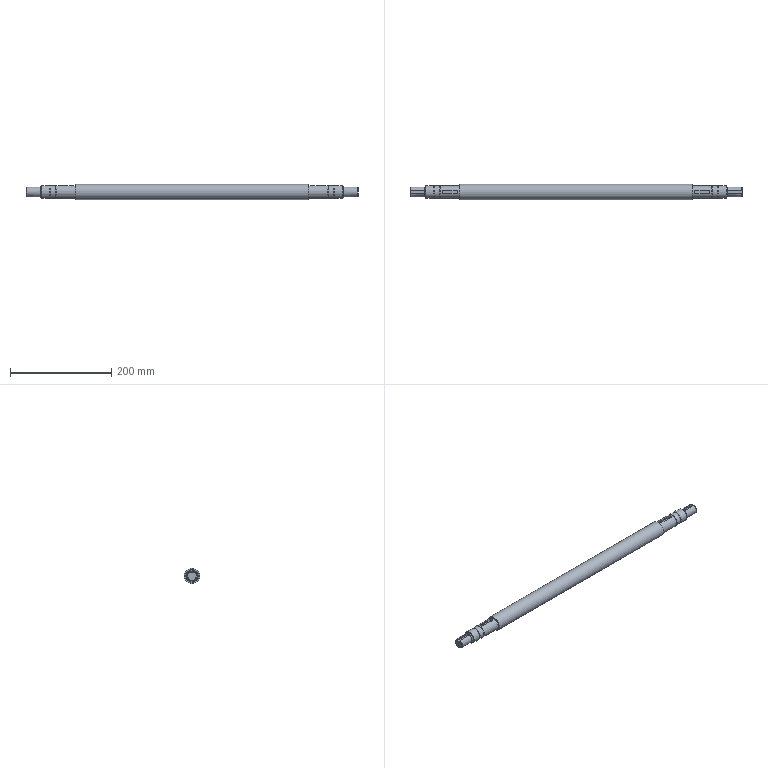NC program | NX | posted with a generic post | part box 656 x 30.5 x 30.5 mm
Lines 1907 to 2071 of 2071:
(ZLEVEL_PROFILE_COPY_COPY , TOOL : D4JING)
N3806 T05 M6
N3808 G54
N3810 G17 G0 G90 X332.554 Y0. S5000 M3
N3812 G43 Z30. H5
N3814 Z-7.75
N3816 G94 G1 Z-8.75 F1000.
N3818 X331.184 Y0.252
N3820 G3 X330.75 Y0.5 R0.5
N3822 G1 X330.48 Y0.499
N3824 X328.24 Y0.498
N3826 X328. Y0.5
N3828 X302.
N3830 G3 X301.5 Y0. R0.5
N3832 X302. Y-0.5 R0.5
N3834 G1 X328.
N3836 X328.318 Y-0.499
N3838 X330.48
N3840 X330.75 Y-0.5
N3842 G3 X331.184 Y-0.252 R0.5
N3844 G1 X332.554 Y0.
N3846 Z-7.75
N3848 G0 Z30.
N3850 X-332.553
N3852 Z-7.75
N3854 G1 Z-8.75
N3856 X-331.183 Y-0.25
N3858 G3 X-330.749 Y-0.5 R0.5
N3860 G1 X-327.965 Y-0.499
N3862 X-327.65 Y-0.5
N3864 X-302.
N3866 G3 X-301.5 Y0. R0.5
N3868 X-302. Y0.5 R0.5
N3870 G1 X-327.65
N3872 X-330.749
N3874 G3 X-331.182 Y0.25 R0.5
N3876 G1 X-332.553 Y0.
N3878 Z-7.75
N3880 G0 Z30.
(ZLEVEL_PROFILE_COPY_COPY_COPY , TOOL : D4JING)
N3882 X-236.75
N3884 Z-4.75
N3886 G1 Z-5.75
N3888 X-236.317 Y0.25
N3890 G3 X-236.75 Y0.5 R0.5
N3892 G1 X-261.75
N3894 G3 X-262.25 Y0. R0.5
N3896 X-261.75 Y-0.5 R0.5
N3898 G1 X-236.75
N3900 G3 X-236.25 Y0. R0.5
N3902 X-236.75 Y0.5 R0.5
N3904 X-237.183 Y0.25 R0.5
N3906 G1 X-237.327 Y0.
N3908 Z-4.75
N3910 G0 Z30.
N3912 X261.75
N3914 Z-4.75
N3916 G1 Z-5.75
N3918 X262.183 Y0.25
N3920 G3 X261.75 Y0.5 R0.5
N3922 G1 X236.75
N3924 G3 X236.25 Y0. R0.5
N3926 X236.75 Y-0.5 R0.5
N3928 G1 X261.75
N3930 G3 X262.25 Y0. R0.5
N3932 X261.75 Y0.5 R0.5
N3934 X261.317 Y0.25 R0.5
N3936 G1 X261.173 Y0.
N3938 Z-4.75
N3940 G0 Z30.
N3942 M5
(ZLEVEL_PROFILE_1_COPY_1_COPY , TOOL : D6A45)
N3944 T02 M6
N3946 G54
N3948 G17 G0 G90 X261.835 Y0.779 S7500 M3
N3950 G43 Z30. H2
N3952 Z-3.
N3954 G94 G1 Z-4. F1000.
N3956 X262.182 Y1.703
N3958 G3 X261.663 Y2.003 R0.6
N3960 G1 X236.837
N3962 G3 X235.429 Y1.21 R1.575
N3964 X235.429 Y-1.21 R2.415
N3966 X236.837 Y-2.003 R1.574
N3968 G1 X261.663
N3970 G3 X263.071 Y-1.21 R1.575
N3972 X263.071 Y1.21 R2.415
N3974 X261.663 Y2.003 R1.574
N3976 X261.151 Y1.689 R0.6
N3978 G1 X260.67 Y0.803
N3980 Z-3.
N3982 G0 Z30.
N3984 X-236.665 Y0.779
N3986 Z-3.
N3988 G1 Z-4.
N3990 X-236.318 Y1.703
N3992 G3 X-236.837 Y2.003 R0.6
N3994 G1 X-261.663
N3996 G3 X-263.071 Y1.21 R1.574
N3998 X-263.071 Y-1.21 R2.415
N4000 X-261.663 Y-2.003 R1.575
N4002 G1 X-236.837
N4004 G3 X-235.429 Y-1.21 R1.574
N4006 X-235.429 Y1.21 R2.415
N4008 X-236.837 Y2.003 R1.575
N4010 X-237.349 Y1.689 R0.6
N4012 G1 X-237.83 Y0.803
N4014 Z-3.
N4016 G0 Z30.
(ZLEVEL_PROFILE_1_COPY_1_COPY_COPY , TOOL : D6A45)
N4018 X329.039 Y0.445
N4020 Z-6.473
N4022 G1 Z-7.473
N4024 X328.52 Y1.345
N4026 G3 X328. Y1.645 R0.6
N4028 G1 X302.153
N4030 X302.031 Y1.642
N4032 G3 X301.237 Y1.297 R1.166
N4034 X301.16 Y1.007 R0.3
N4036 G1 X302.075 Y0.439
N4038 Z-6.473
N4040 G0 Z30.
N4042 X302.073 Y-0.437
N4044 Z-6.473
N4046 G1 Z-7.473
N4048 X301.16 Y-1.007
N4050 G3 X301.237 Y-1.297 R0.3
N4052 X302.073 Y-1.645 R1.18
N4054 G1 X328.
N4056 G3 X328.52 Y-1.345 R0.6
N4058 G1 X329.039 Y-0.445
N4060 Z-6.473
N4062 G0 Z30.
N4064 X-329.039 Y-0.446
N4066 Z-6.473
N4068 G1 Z-7.473
N4070 X-328.52 Y-1.346
N4072 G3 X-328. Y-1.646 R0.6
N4074 G1 X-302.073 Y-1.645
N4076 G3 X-301.237 Y-1.297 R1.18
N4078 X-301.16 Y-1.007 R0.3
N4080 G1 X-302.017 Y-0.385
N4082 Z-6.473
N4084 G0 Z30.
N4086 X-302.023 Y0.389
N4088 Z-6.473
N4090 G1 Z-7.473
N4092 X-301.16 Y1.007
N4094 G3 X-301.237 Y1.297 R0.3
N4096 X-302.073 Y1.645 R1.18
N4098 G1 X-328. Y1.646
N4100 G3 X-328.52 Y1.346 R0.6
N4102 G1 X-329.039 Y0.446
N4104 Z-6.473
N4106 G0 Z30.
N4108 M5
N4110 M2